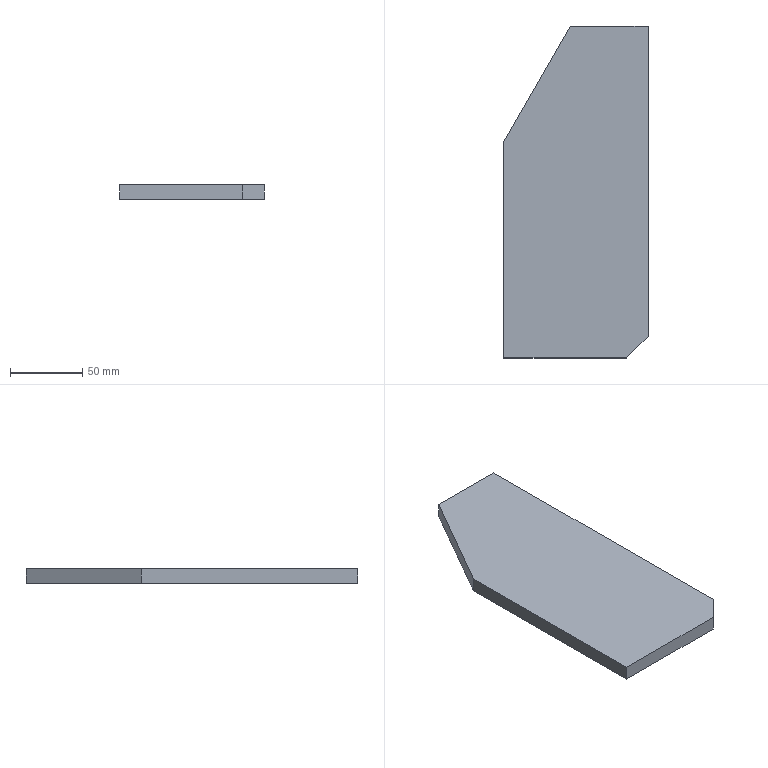Part | SolidWorks | features Chamfer 1, Extrusion 1 | 1 solid | 8 faces | box 100 x 230 x 10 mm | volume 210475 mm3 | plane 8
STEP:
#1=CARTESIAN_POINT('',(0.,0.,-5.));
#2=VERTEX_POINT('',#1);
#3=CARTESIAN_POINT('',(85.,0.,-5.));
#4=VERTEX_POINT('',#3);
#5=CARTESIAN_POINT('',(100.,0.,-5.));
#6=DIRECTION('',(1.,0.,0.));
#7=VECTOR('',#6,1000.);
#8=LINE('',#5,#7);
#9=EDGE_CURVE('',#2,#4,#8,.T.);
#10=ORIENTED_EDGE('',*,*,#9,.T.);
#11=CARTESIAN_POINT('',(85.,0.,5.));
#12=VERTEX_POINT('',#11);
#13=CARTESIAN_POINT('',(85.,0.,5.));
#14=DIRECTION('',(0.,0.,1.));
#15=VECTOR('',#14,1000.);
#16=LINE('',#13,#15);
#17=EDGE_CURVE('',#4,#12,#16,.T.);
#18=ORIENTED_EDGE('',*,*,#17,.T.);
#19=CARTESIAN_POINT('',(0.,0.,5.));
#20=VERTEX_POINT('',#19);
#21=CARTESIAN_POINT('',(100.,0.,5.));
#22=DIRECTION('',(1.,0.,0.));
#23=VECTOR('',#22,1000.);
#24=LINE('',#21,#23);
#25=EDGE_CURVE('',#20,#12,#24,.T.);
#26=ORIENTED_EDGE('',*,*,#25,.F.);
#27=CARTESIAN_POINT('',(0.,0.,5.));
#28=DIRECTION('',(0.,0.,-1.));
#29=VECTOR('',#28,1000.);
#30=LINE('',#27,#29);
#31=EDGE_CURVE('',#20,#2,#30,.T.);
#32=ORIENTED_EDGE('',*,*,#31,.T.);
#33=EDGE_LOOP('',(#10,#18,#26,#32));
#34=FACE_OUTER_BOUND('',#33,.T.);
#35=CARTESIAN_POINT('',(100.,0.,5.));
#36=DIRECTION('',(0.,1.,0.));
#37=DIRECTION('',(0.,0.,1.));
#38=AXIS2_PLACEMENT_3D('',#35,#36,#37);
#39=PLANE('',#38);
#40=ADVANCED_FACE('',(#34),#39,.F.);
#41=CARTESIAN_POINT('',(100.,15.,5.));
#42=VERTEX_POINT('',#41);
#43=CARTESIAN_POINT('',(100.,230.,5.));
#44=VERTEX_POINT('',#43);
#45=CARTESIAN_POINT('',(100.,230.,5.));
#46=DIRECTION('',(0.,1.,0.));
#47=VECTOR('',#46,1000.);
#48=LINE('',#45,#47);
#49=EDGE_CURVE('',#42,#44,#48,.T.);
#50=ORIENTED_EDGE('',*,*,#49,.F.);
#51=CARTESIAN_POINT('',(100.,15.,-5.));
#52=VERTEX_POINT('',#51);
#53=CARTESIAN_POINT('',(100.,15.,5.));
#54=DIRECTION('',(0.,0.,-1.));
#55=VECTOR('',#54,1000.);
#56=LINE('',#53,#55);
#57=EDGE_CURVE('',#42,#52,#56,.T.);
#58=ORIENTED_EDGE('',*,*,#57,.T.);
#59=CARTESIAN_POINT('',(100.,230.,-5.));
#60=VERTEX_POINT('',#59);
#61=CARTESIAN_POINT('',(100.,230.,-5.));
#62=DIRECTION('',(0.,1.,0.));
#63=VECTOR('',#62,1000.);
#64=LINE('',#61,#63);
#65=EDGE_CURVE('',#52,#60,#64,.T.);
#66=ORIENTED_EDGE('',*,*,#65,.T.);
#67=CARTESIAN_POINT('',(100.,230.,5.));
#68=DIRECTION('',(0.,0.,-1.));
#69=VECTOR('',#68,1000.);
#70=LINE('',#67,#69);
#71=EDGE_CURVE('',#44,#60,#70,.T.);
#72=ORIENTED_EDGE('',*,*,#71,.F.);
#73=EDGE_LOOP('',(#50,#58,#66,#72));
#74=FACE_OUTER_BOUND('',#73,.T.);
#75=CARTESIAN_POINT('',(100.,230.,5.));
#76=DIRECTION('',(-1.,0.,0.));
#77=DIRECTION('',(0.,-1.,0.));
#78=AXIS2_PLACEMENT_3D('',#75,#76,#77);
#79=PLANE('',#78);
#80=ADVANCED_FACE('',(#74),#79,.F.);
#81=CARTESIAN_POINT('',(46.,230.,-5.));
#82=VERTEX_POINT('',#81);
#83=CARTESIAN_POINT('',(46.,230.,-5.));
#84=DIRECTION('',(-1.,0.,0.));
#85=VECTOR('',#84,1000.);
#86=LINE('',#83,#85);
#87=EDGE_CURVE('',#60,#82,#86,.T.);
#88=ORIENTED_EDGE('',*,*,#87,.T.);
#89=CARTESIAN_POINT('',(46.,230.,5.));
#90=VERTEX_POINT('',#89);
#91=CARTESIAN_POINT('',(46.,230.,5.));
#92=DIRECTION('',(0.,0.,-1.));
#93=VECTOR('',#92,1000.);
#94=LINE('',#91,#93);
#95=EDGE_CURVE('',#90,#82,#94,.T.);
#96=ORIENTED_EDGE('',*,*,#95,.F.);
#97=CARTESIAN_POINT('',(46.,230.,5.));
#98=DIRECTION('',(-1.,0.,0.));
#99=VECTOR('',#98,1000.);
#100=LINE('',#97,#99);
#101=EDGE_CURVE('',#44,#90,#100,.T.);
#102=ORIENTED_EDGE('',*,*,#101,.F.);
#103=ORIENTED_EDGE('',*,*,#71,.T.);
#104=EDGE_LOOP('',(#88,#96,#102,#103));
#105=FACE_OUTER_BOUND('',#104,.T.);
#106=CARTESIAN_POINT('',(46.,230.,5.));
#107=DIRECTION('',(0.,-1.,0.));
#108=DIRECTION('',(0.,0.,-1.));
#109=AXIS2_PLACEMENT_3D('',#106,#107,#108);
#110=PLANE('',#109);
#111=ADVANCED_FACE('',(#105),#110,.F.);
#112=CARTESIAN_POINT('',(0.,150.,-5.));
#113=VERTEX_POINT('',#112);
#114=CARTESIAN_POINT('',(0.,150.,-5.));
#115=DIRECTION('',(-0.4985,-0.8669,0.));
#116=VECTOR('',#115,1000.);
#117=LINE('',#114,#116);
#118=EDGE_CURVE('',#82,#113,#117,.T.);
#119=ORIENTED_EDGE('',*,*,#118,.T.);
#120=CARTESIAN_POINT('',(0.,150.,5.));
#121=VERTEX_POINT('',#120);
#122=CARTESIAN_POINT('',(0.,150.,5.));
#123=DIRECTION('',(0.,0.,-1.));
#124=VECTOR('',#123,1000.);
#125=LINE('',#122,#124);
#126=EDGE_CURVE('',#121,#113,#125,.T.);
#127=ORIENTED_EDGE('',*,*,#126,.F.);
#128=CARTESIAN_POINT('',(0.,150.,5.));
#129=DIRECTION('',(-0.4985,-0.8669,0.));
#130=VECTOR('',#129,1000.);
#131=LINE('',#128,#130);
#132=EDGE_CURVE('',#90,#121,#131,.T.);
#133=ORIENTED_EDGE('',*,*,#132,.F.);
#134=ORIENTED_EDGE('',*,*,#95,.T.);
#135=EDGE_LOOP('',(#119,#127,#133,#134));
#136=FACE_OUTER_BOUND('',#135,.T.);
#137=CARTESIAN_POINT('',(0.,150.,5.));
#138=DIRECTION('',(0.8669,-0.4985,0.));
#139=DIRECTION('',(0.4985,0.8669,0.));
#140=AXIS2_PLACEMENT_3D('',#137,#138,#139);
#141=PLANE('',#140);
#142=ADVANCED_FACE('',(#136),#141,.F.);
#143=CARTESIAN_POINT('',(0.,0.,-5.));
#144=DIRECTION('',(0.,-1.,0.));
#145=VECTOR('',#144,1000.);
#146=LINE('',#143,#145);
#147=EDGE_CURVE('',#113,#2,#146,.T.);
#148=ORIENTED_EDGE('',*,*,#147,.T.);
#149=ORIENTED_EDGE('',*,*,#31,.F.);
#150=CARTESIAN_POINT('',(0.,0.,5.));
#151=DIRECTION('',(0.,-1.,0.));
#152=VECTOR('',#151,1000.);
#153=LINE('',#150,#152);
#154=EDGE_CURVE('',#121,#20,#153,.T.);
#155=ORIENTED_EDGE('',*,*,#154,.F.);
#156=ORIENTED_EDGE('',*,*,#126,.T.);
#157=EDGE_LOOP('',(#148,#149,#155,#156));
#158=FACE_OUTER_BOUND('',#157,.T.);
#159=CARTESIAN_POINT('',(0.,0.,5.));
#160=DIRECTION('',(1.,0.,0.));
#161=DIRECTION('',(0.,0.,-1.));
#162=AXIS2_PLACEMENT_3D('',#159,#160,#161);
#163=PLANE('',#162);
#164=ADVANCED_FACE('',(#158),#163,.F.);
#165=ORIENTED_EDGE('',*,*,#25,.T.);
#166=CARTESIAN_POINT('',(100.,15.,5.));
#167=DIRECTION('',(0.7071,0.7071,0.));
#168=VECTOR('',#167,1000.);
#169=LINE('',#166,#168);
#170=EDGE_CURVE('',#12,#42,#169,.T.);
#171=ORIENTED_EDGE('',*,*,#170,.T.);
#172=ORIENTED_EDGE('',*,*,#49,.T.);
#173=ORIENTED_EDGE('',*,*,#101,.T.);
#174=ORIENTED_EDGE('',*,*,#132,.T.);
#175=ORIENTED_EDGE('',*,*,#154,.T.);
#176=EDGE_LOOP('',(#165,#171,#172,#173,#174,#175));
#177=FACE_OUTER_BOUND('',#176,.T.);
#178=CARTESIAN_POINT('',(0.,0.,5.));
#179=DIRECTION('',(0.,0.,-1.));
#180=DIRECTION('',(-1.,0.,0.));
#181=AXIS2_PLACEMENT_3D('',#178,#179,#180);
#182=PLANE('',#181);
#183=ADVANCED_FACE('',(#177),#182,.F.);
#184=ORIENTED_EDGE('',*,*,#65,.F.);
#185=CARTESIAN_POINT('',(42.5,-42.5,-5.));
#186=DIRECTION('',(-0.7071,-0.7071,0.));
#187=VECTOR('',#186,1000.);
#188=LINE('',#185,#187);
#189=EDGE_CURVE('',#52,#4,#188,.T.);
#190=ORIENTED_EDGE('',*,*,#189,.T.);
#191=ORIENTED_EDGE('',*,*,#9,.F.);
#192=ORIENTED_EDGE('',*,*,#147,.F.);
#193=ORIENTED_EDGE('',*,*,#118,.F.);
#194=ORIENTED_EDGE('',*,*,#87,.F.);
#195=EDGE_LOOP('',(#184,#190,#191,#192,#193,#194));
#196=FACE_OUTER_BOUND('',#195,.T.);
#197=CARTESIAN_POINT('',(0.,0.,-5.));
#198=DIRECTION('',(0.,0.,-1.));
#199=DIRECTION('',(-1.,0.,0.));
#200=AXIS2_PLACEMENT_3D('',#197,#198,#199);
#201=PLANE('',#200);
#202=ADVANCED_FACE('',(#196),#201,.T.);
#203=ORIENTED_EDGE('',*,*,#170,.F.);
#204=ORIENTED_EDGE('',*,*,#17,.F.);
#205=ORIENTED_EDGE('',*,*,#189,.F.);
#206=ORIENTED_EDGE('',*,*,#57,.F.);
#207=EDGE_LOOP('',(#203,#204,#205,#206));
#208=FACE_OUTER_BOUND('',#207,.T.);
#209=CARTESIAN_POINT('',(100.,15.,5.));
#210=DIRECTION('',(-0.7071,0.7071,0.));
#211=DIRECTION('',(0.,0.,-1.));
#212=AXIS2_PLACEMENT_3D('',#209,#210,#211);
#213=PLANE('',#212);
#214=ADVANCED_FACE('',(#208),#213,.F.);
#215=CLOSED_SHELL('',(#40,#80,#111,#142,#164,#183,#202,#214));
#216=MANIFOLD_SOLID_BREP('',#215);
#217=CARTESIAN_POINT('',(0.,0.,0.));
#218=DIRECTION('',(0.,0.,1.));
#219=DIRECTION('',(1.,0.,0.));
#220=AXIS2_PLACEMENT_3D('',#217,#218,#219);
#221=(LENGTH_UNIT()NAMED_UNIT(*)SI_UNIT(.MILLI.,.METRE.));
#222=UNCERTAINTY_MEASURE_WITH_UNIT(LENGTH_MEASURE(0.00001),#221,'','');
#223=(NAMED_UNIT(*)PLANE_ANGLE_UNIT()SI_UNIT($,.RADIAN.));
#224=(NAMED_UNIT(*)SI_UNIT($,.STERADIAN.)SOLID_ANGLE_UNIT());
#225=(GEOMETRIC_REPRESENTATION_CONTEXT(3)GLOBAL_UNCERTAINTY_ASSIGNED_CONTEXT((#222))GLOBAL_UNIT_ASSIGNED_CONTEXT((#221,#223,#224))REPRESENTATION_CONTEXT('',''));
#226=ADVANCED_BREP_SHAPE_REPRESENTATION('',(#216,#220),#225);